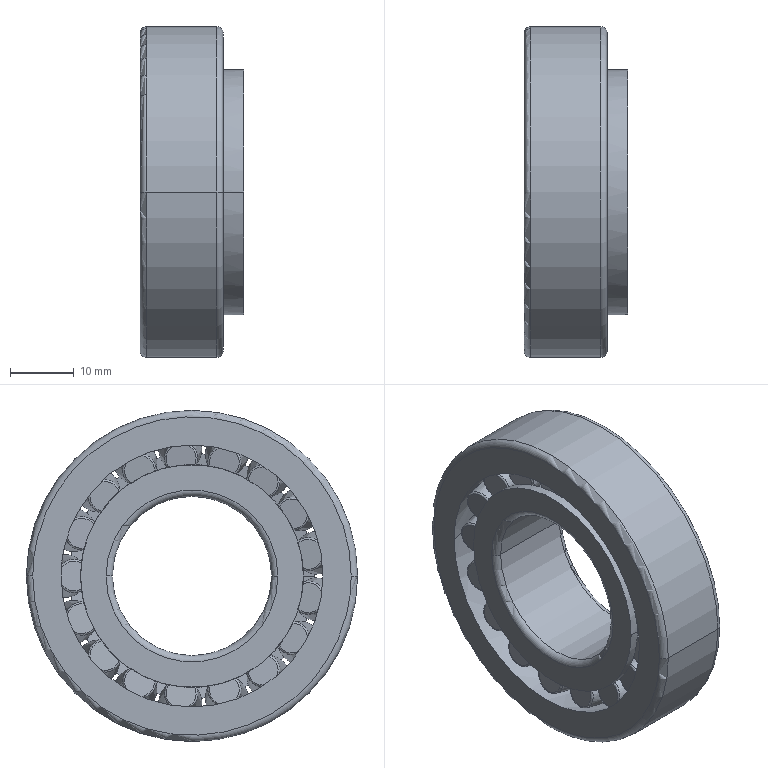Part | STEP file | PN_0038_Default<As Machined> | 1 solid | 198 faces | box 16.25 x 52 x 52 mm | volume 18571 mm3 | torus 110 | cone 42 | plane 38 | cylinder 8 | commonest cylinder face diameters 25 x2 34.984 x2 38.5 x2 52 x2